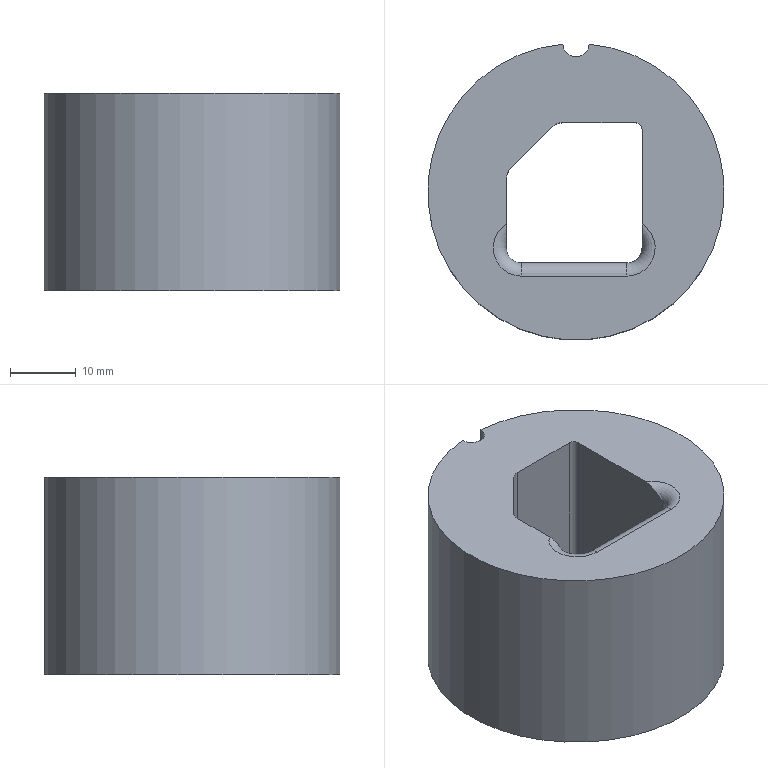Part | NX | features 23 2 | 1 solid | 17 faces | box 45 x 44.911 x 30 mm | volume 35277 mm3 | cylinder 8 | plane 7 | torus 2 | commonest cylinder face diameters 4.6 x4 2 x1 4 x1 4.001 x1 45 x1
STEP:
#1=CARTESIAN_POINT('',(147.222,-436.51,-33.5));
#2=VERTEX_POINT('',#1);
#3=CARTESIAN_POINT('',(144.922,-438.81,-33.5));
#4=VERTEX_POINT('',#3);
#5=CARTESIAN_POINT('',(144.922,-436.51,-33.5));
#6=DIRECTION('',(0.,0.,-1.));
#7=DIRECTION('',(-1.,0.,0.));
#8=AXIS2_PLACEMENT_3D('',#5,#6,#7);
#9=CIRCLE('',#8,2.3);
#10=EDGE_CURVE('',#2,#4,#9,.T.);
#11=ORIENTED_EDGE('',*,*,#10,.F.);
#12=CARTESIAN_POINT('',(147.222,-418.5,-33.5));
#13=VERTEX_POINT('',#12);
#14=CARTESIAN_POINT('',(147.222,-377.506,-33.5));
#15=DIRECTION('',(0.,1.,0.));
#16=VECTOR('',#15,1000.);
#17=LINE('',#14,#16);
#18=EDGE_CURVE('',#2,#13,#17,.T.);
#19=ORIENTED_EDGE('',*,*,#18,.T.);
#20=CARTESIAN_POINT('',(146.222,-417.5,-33.5));
#21=VERTEX_POINT('',#20);
#22=CARTESIAN_POINT('',(146.222,-418.5,-33.5));
#23=DIRECTION('',(0.,0.,1.));
#24=DIRECTION('',(-1.,0.,0.));
#25=AXIS2_PLACEMENT_3D('',#22,#23,#24);
#26=CIRCLE('',#25,1.);
#27=EDGE_CURVE('',#13,#21,#26,.T.);
#28=ORIENTED_EDGE('',*,*,#27,.T.);
#29=CARTESIAN_POINT('',(135.152,-417.5,-33.5));
#30=VERTEX_POINT('',#29);
#31=CARTESIAN_POINT('',(119.455,-417.5,-33.5));
#32=DIRECTION('',(-1.,0.,0.));
#33=VECTOR('',#32,1000.);
#34=LINE('',#31,#33);
#35=EDGE_CURVE('',#21,#30,#34,.T.);
#36=ORIENTED_EDGE('',*,*,#35,.T.);
#37=CARTESIAN_POINT('',(133.525,-418.174,-33.5));
#38=VERTEX_POINT('',#37);
#39=CARTESIAN_POINT('',(135.152,-419.8,-33.5));
#40=DIRECTION('',(0.,0.,1.));
#41=DIRECTION('',(-1.,0.,0.));
#42=AXIS2_PLACEMENT_3D('',#39,#40,#41);
#43=CIRCLE('',#42,2.3);
#44=EDGE_CURVE('',#30,#38,#43,.T.);
#45=ORIENTED_EDGE('',*,*,#44,.T.);
#46=CARTESIAN_POINT('',(127.295,-424.404,-33.5));
#47=VERTEX_POINT('',#46);
#48=CARTESIAN_POINT('',(146.824,-404.875,-33.5));
#49=DIRECTION('',(-0.7071,-0.7071,0.));
#50=VECTOR('',#49,1000.);
#51=LINE('',#48,#50);
#52=EDGE_CURVE('',#38,#47,#51,.T.);
#53=ORIENTED_EDGE('',*,*,#52,.T.);
#54=CARTESIAN_POINT('',(126.622,-426.03,-33.5));
#55=VERTEX_POINT('',#54);
#56=CARTESIAN_POINT('',(128.922,-426.03,-33.5));
#57=DIRECTION('',(0.,0.,1.));
#58=DIRECTION('',(-1.,0.,0.));
#59=AXIS2_PLACEMENT_3D('',#56,#57,#58);
#60=CIRCLE('',#59,2.3);
#61=EDGE_CURVE('',#47,#55,#60,.T.);
#62=ORIENTED_EDGE('',*,*,#61,.T.);
#63=CARTESIAN_POINT('',(126.622,-436.51,-33.5));
#64=VERTEX_POINT('',#63);
#65=CARTESIAN_POINT('',(126.622,-377.506,-33.5));
#66=DIRECTION('',(0.,-1.,0.));
#67=VECTOR('',#66,1000.);
#68=LINE('',#65,#67);
#69=EDGE_CURVE('',#55,#64,#68,.T.);
#70=ORIENTED_EDGE('',*,*,#69,.T.);
#71=CARTESIAN_POINT('',(128.922,-438.81,-33.5));
#72=VERTEX_POINT('',#71);
#73=CARTESIAN_POINT('',(128.922,-436.51,-33.5));
#74=DIRECTION('',(0.,0.,-1.));
#75=DIRECTION('',(-1.,0.,0.));
#76=AXIS2_PLACEMENT_3D('',#73,#74,#75);
#77=CIRCLE('',#76,2.3);
#78=EDGE_CURVE('',#72,#64,#77,.T.);
#79=ORIENTED_EDGE('',*,*,#78,.F.);
#80=CARTESIAN_POINT('',(119.455,-438.81,-33.5));
#81=DIRECTION('',(1.,0.,0.));
#82=VECTOR('',#81,1000.);
#83=LINE('',#80,#82);
#84=EDGE_CURVE('',#72,#4,#83,.T.);
#85=ORIENTED_EDGE('',*,*,#84,.T.);
#86=EDGE_LOOP('',(#11,#19,#28,#36,#45,#53,#62,#70,#79,#85));
#87=FACE_BOUND('',#86,.T.);
#88=CARTESIAN_POINT('',(139.198,-405.589,-33.5));
#89=VERTEX_POINT('',#88);
#90=CARTESIAN_POINT('',(135.201,-405.589,-33.5));
#91=VERTEX_POINT('',#90);
#92=CARTESIAN_POINT('',(137.199,-428.,-33.5));
#93=DIRECTION('',(0.,0.,-1.));
#94=DIRECTION('',(-1.,0.,0.));
#95=AXIS2_PLACEMENT_3D('',#92,#93,#94);
#96=CIRCLE('',#95,22.5);
#97=EDGE_CURVE('',#89,#91,#96,.T.);
#98=ORIENTED_EDGE('',*,*,#97,.T.);
#99=CARTESIAN_POINT('',(137.199,-405.5,-33.5));
#100=DIRECTION('',(0.,0.,1.));
#101=DIRECTION('',(1.,0.,0.));
#102=AXIS2_PLACEMENT_3D('',#99,#100,#101);
#103=CIRCLE('',#102,2.001);
#104=EDGE_CURVE('',#91,#89,#103,.T.);
#105=ORIENTED_EDGE('',*,*,#104,.T.);
#106=EDGE_LOOP('',(#98,#105));
#107=FACE_BOUND('',#106,.T.);
#108=CARTESIAN_POINT('',(119.455,-377.506,-33.5));
#109=DIRECTION('',(0.,0.,-1.));
#110=DIRECTION('',(-1.,0.,0.));
#111=AXIS2_PLACEMENT_3D('',#108,#109,#110);
#112=PLANE('',#111);
#113=ADVANCED_FACE('',(#87,#107),#112,.T.);
#114=CARTESIAN_POINT('',(135.201,-405.589,-3.5));
#115=VERTEX_POINT('',#114);
#116=CARTESIAN_POINT('',(139.198,-405.589,-3.5));
#117=VERTEX_POINT('',#116);
#118=CARTESIAN_POINT('',(137.199,-428.,-3.5));
#119=DIRECTION('',(0.,0.,1.));
#120=DIRECTION('',(-1.,0.,0.));
#121=AXIS2_PLACEMENT_3D('',#118,#119,#120);
#122=CIRCLE('',#121,22.5);
#123=EDGE_CURVE('',#115,#117,#122,.T.);
#124=ORIENTED_EDGE('',*,*,#123,.F.);
#125=CARTESIAN_POINT('',(135.201,-405.589,66.5));
#126=DIRECTION('',(0.,0.,-1.));
#127=VECTOR('',#126,1000.);
#128=LINE('',#125,#127);
#129=EDGE_CURVE('',#115,#91,#128,.T.);
#130=ORIENTED_EDGE('',*,*,#129,.T.);
#131=ORIENTED_EDGE('',*,*,#97,.F.);
#132=CARTESIAN_POINT('',(139.198,-405.589,66.5));
#133=DIRECTION('',(0.,0.,1.));
#134=VECTOR('',#133,1000.);
#135=LINE('',#132,#134);
#136=EDGE_CURVE('',#89,#117,#135,.T.);
#137=ORIENTED_EDGE('',*,*,#136,.T.);
#138=EDGE_LOOP('',(#124,#130,#131,#137));
#139=FACE_BOUND('',#138,.T.);
#140=CARTESIAN_POINT('',(137.199,-428.,-158.));
#141=DIRECTION('',(0.,0.,1.));
#142=DIRECTION('',(-1.,0.,0.));
#143=AXIS2_PLACEMENT_3D('',#140,#141,#142);
#144=CYLINDRICAL_SURFACE('',#143,22.5);
#145=ADVANCED_FACE('',(#139),#144,.T.);
#146=CARTESIAN_POINT('',(147.222,-436.51,-5.5));
#147=VERTEX_POINT('',#146);
#148=CARTESIAN_POINT('',(147.222,-436.51,210.5));
#149=DIRECTION('',(0.,0.,1.));
#150=VECTOR('',#149,1000.);
#151=LINE('',#148,#150);
#152=EDGE_CURVE('',#2,#147,#151,.T.);
#153=ORIENTED_EDGE('',*,*,#152,.T.);
#154=CARTESIAN_POINT('',(147.222,-432.877,-3.5));
#155=VERTEX_POINT('',#154);
#156=CARTESIAN_POINT('',(147.222,-436.51,-5.5));
#157=CARTESIAN_POINT('',(147.222,-435.992,-5.017));
#158=CARTESIAN_POINT('',(147.222,-434.95,-4.041));
#159=CARTESIAN_POINT('',(147.222,-433.59,-3.5));
#160=CARTESIAN_POINT('',(147.222,-432.877,-3.5));
#161=B_SPLINE_CURVE_WITH_KNOTS('',3,(#156,#157,#158,#159,#160),.UNSPECIFIED.,.F.,.F.,(4,1,4),(-0.000009592,0.002115,0.004239),.UNSPECIFIED.);
#162=EDGE_CURVE('',#147,#155,#161,.T.);
#163=ORIENTED_EDGE('',*,*,#162,.T.);
#164=CARTESIAN_POINT('',(147.222,-418.5,-3.5));
#165=VERTEX_POINT('',#164);
#166=CARTESIAN_POINT('',(147.222,-384.125,-3.5));
#167=DIRECTION('',(0.,-1.,0.));
#168=VECTOR('',#167,1000.);
#169=LINE('',#166,#168);
#170=EDGE_CURVE('',#165,#155,#169,.T.);
#171=ORIENTED_EDGE('',*,*,#170,.F.);
#172=CARTESIAN_POINT('',(147.222,-418.5,210.5));
#173=DIRECTION('',(0.,0.,1.));
#174=VECTOR('',#173,1000.);
#175=LINE('',#172,#174);
#176=EDGE_CURVE('',#13,#165,#175,.T.);
#177=ORIENTED_EDGE('',*,*,#176,.F.);
#178=ORIENTED_EDGE('',*,*,#18,.F.);
#179=EDGE_LOOP('',(#153,#163,#171,#177,#178));
#180=FACE_BOUND('',#179,.T.);
#181=CARTESIAN_POINT('',(147.222,-384.125,210.5));
#182=DIRECTION('',(-1.,0.,0.));
#183=DIRECTION('',(0.,0.,1.));
#184=AXIS2_PLACEMENT_3D('',#181,#182,#183);
#185=PLANE('',#184);
#186=ADVANCED_FACE('',(#180),#185,.T.);
#187=CARTESIAN_POINT('',(146.222,-417.5,-3.5));
#188=VERTEX_POINT('',#187);
#189=CARTESIAN_POINT('',(146.222,-417.5,210.5));
#190=DIRECTION('',(0.,0.,1.));
#191=VECTOR('',#190,1000.);
#192=LINE('',#189,#191);
#193=EDGE_CURVE('',#21,#188,#192,.T.);
#194=ORIENTED_EDGE('',*,*,#193,.F.);
#195=ORIENTED_EDGE('',*,*,#27,.F.);
#196=ORIENTED_EDGE('',*,*,#176,.T.);
#197=CARTESIAN_POINT('',(146.222,-418.5,-3.5));
#198=DIRECTION('',(0.,0.,-1.));
#199=DIRECTION('',(-1.,0.,0.));
#200=AXIS2_PLACEMENT_3D('',#197,#198,#199);
#201=CIRCLE('',#200,1.);
#202=EDGE_CURVE('',#188,#165,#201,.T.);
#203=ORIENTED_EDGE('',*,*,#202,.F.);
#204=EDGE_LOOP('',(#194,#195,#196,#203));
#205=FACE_BOUND('',#204,.T.);
#206=CARTESIAN_POINT('',(146.222,-418.5,210.5));
#207=DIRECTION('',(0.,0.,-1.));
#208=DIRECTION('',(1.,0.,0.));
#209=AXIS2_PLACEMENT_3D('',#206,#207,#208);
#210=CYLINDRICAL_SURFACE('',#209,1.);
#211=ADVANCED_FACE('',(#205),#210,.F.);
#212=CARTESIAN_POINT('',(135.152,-417.5,-3.5));
#213=VERTEX_POINT('',#212);
#214=CARTESIAN_POINT('',(135.152,-417.5,210.5));
#215=DIRECTION('',(0.,0.,1.));
#216=VECTOR('',#215,1000.);
#217=LINE('',#214,#216);
#218=EDGE_CURVE('',#30,#213,#217,.T.);
#219=ORIENTED_EDGE('',*,*,#218,.F.);
#220=ORIENTED_EDGE('',*,*,#35,.F.);
#221=ORIENTED_EDGE('',*,*,#193,.T.);
#222=CARTESIAN_POINT('',(205.494,-417.5,-3.5));
#223=DIRECTION('',(1.,0.,0.));
#224=VECTOR('',#223,1000.);
#225=LINE('',#222,#224);
#226=EDGE_CURVE('',#213,#188,#225,.T.);
#227=ORIENTED_EDGE('',*,*,#226,.F.);
#228=EDGE_LOOP('',(#219,#220,#221,#227));
#229=FACE_BOUND('',#228,.T.);
#230=CARTESIAN_POINT('',(205.494,-417.5,210.5));
#231=DIRECTION('',(0.,-1.,0.));
#232=DIRECTION('',(0.,0.,-1.));
#233=AXIS2_PLACEMENT_3D('',#230,#231,#232);
#234=PLANE('',#233);
#235=ADVANCED_FACE('',(#229),#234,.T.);
#236=CARTESIAN_POINT('',(133.525,-418.174,-3.5));
#237=VERTEX_POINT('',#236);
#238=CARTESIAN_POINT('',(133.525,-418.174,-48.5));
#239=DIRECTION('',(0.,0.,1.));
#240=VECTOR('',#239,1000.);
#241=LINE('',#238,#240);
#242=EDGE_CURVE('',#38,#237,#241,.T.);
#243=ORIENTED_EDGE('',*,*,#242,.F.);
#244=ORIENTED_EDGE('',*,*,#44,.F.);
#245=ORIENTED_EDGE('',*,*,#218,.T.);
#246=CARTESIAN_POINT('',(135.152,-419.8,-3.5));
#247=DIRECTION('',(0.,0.,-1.));
#248=DIRECTION('',(-1.,0.,0.));
#249=AXIS2_PLACEMENT_3D('',#246,#247,#248);
#250=CIRCLE('',#249,2.3);
#251=EDGE_CURVE('',#237,#213,#250,.T.);
#252=ORIENTED_EDGE('',*,*,#251,.F.);
#253=EDGE_LOOP('',(#243,#244,#245,#252));
#254=FACE_BOUND('',#253,.T.);
#255=CARTESIAN_POINT('',(135.152,-419.8,-48.5));
#256=DIRECTION('',(0.,0.,-1.));
#257=DIRECTION('',(1.,0.,0.));
#258=AXIS2_PLACEMENT_3D('',#255,#256,#257);
#259=CYLINDRICAL_SURFACE('',#258,2.3);
#260=ADVANCED_FACE('',(#254),#259,.F.);
#261=CARTESIAN_POINT('',(127.295,-424.404,-3.5));
#262=VERTEX_POINT('',#261);
#263=CARTESIAN_POINT('',(127.295,-424.404,-48.5));
#264=DIRECTION('',(0.,0.,1.));
#265=VECTOR('',#264,1000.);
#266=LINE('',#263,#265);
#267=EDGE_CURVE('',#47,#262,#266,.T.);
#268=ORIENTED_EDGE('',*,*,#267,.F.);
#269=ORIENTED_EDGE('',*,*,#52,.F.);
#270=ORIENTED_EDGE('',*,*,#242,.T.);
#271=CARTESIAN_POINT('',(127.785,-423.914,-3.5));
#272=DIRECTION('',(0.7071,0.7071,0.));
#273=VECTOR('',#272,1000.);
#274=LINE('',#271,#273);
#275=EDGE_CURVE('',#262,#237,#274,.T.);
#276=ORIENTED_EDGE('',*,*,#275,.F.);
#277=EDGE_LOOP('',(#268,#269,#270,#276));
#278=FACE_BOUND('',#277,.T.);
#279=CARTESIAN_POINT('',(127.785,-423.914,-48.5));
#280=DIRECTION('',(0.7071,-0.7071,0.));
#281=DIRECTION('',(0.7071,0.7071,0.));
#282=AXIS2_PLACEMENT_3D('',#279,#280,#281);
#283=PLANE('',#282);
#284=ADVANCED_FACE('',(#278),#283,.T.);
#285=CARTESIAN_POINT('',(126.622,-426.03,-3.5));
#286=VERTEX_POINT('',#285);
#287=CARTESIAN_POINT('',(126.622,-426.03,210.5));
#288=DIRECTION('',(0.,0.,1.));
#289=VECTOR('',#288,1000.);
#290=LINE('',#287,#289);
#291=EDGE_CURVE('',#55,#286,#290,.T.);
#292=ORIENTED_EDGE('',*,*,#291,.F.);
#293=ORIENTED_EDGE('',*,*,#61,.F.);
#294=ORIENTED_EDGE('',*,*,#267,.T.);
#295=CARTESIAN_POINT('',(128.922,-426.03,-3.5));
#296=DIRECTION('',(0.,0.,-1.));
#297=DIRECTION('',(-1.,0.,0.));
#298=AXIS2_PLACEMENT_3D('',#295,#296,#297);
#299=CIRCLE('',#298,2.3);
#300=EDGE_CURVE('',#286,#262,#299,.T.);
#301=ORIENTED_EDGE('',*,*,#300,.F.);
#302=EDGE_LOOP('',(#292,#293,#294,#301));
#303=FACE_BOUND('',#302,.T.);
#304=CARTESIAN_POINT('',(128.922,-426.03,210.5));
#305=DIRECTION('',(0.,0.,-1.));
#306=DIRECTION('',(1.,0.,0.));
#307=AXIS2_PLACEMENT_3D('',#304,#305,#306);
#308=CYLINDRICAL_SURFACE('',#307,2.3);
#309=ADVANCED_FACE('',(#303),#308,.F.);
#310=CARTESIAN_POINT('',(126.622,-432.877,-3.5));
#311=VERTEX_POINT('',#310);
#312=CARTESIAN_POINT('',(126.622,-384.125,-3.5));
#313=DIRECTION('',(0.,1.,0.));
#314=VECTOR('',#313,1000.);
#315=LINE('',#312,#314);
#316=EDGE_CURVE('',#311,#286,#315,.T.);
#317=ORIENTED_EDGE('',*,*,#316,.F.);
#318=CARTESIAN_POINT('',(126.622,-436.51,-5.5));
#319=VERTEX_POINT('',#318);
#320=CARTESIAN_POINT('',(126.622,-432.877,-3.5));
#321=CARTESIAN_POINT('',(126.622,-433.593,-3.5));
#322=CARTESIAN_POINT('',(126.622,-434.946,-4.04));
#323=CARTESIAN_POINT('',(126.622,-435.993,-5.018));
#324=CARTESIAN_POINT('',(126.622,-436.51,-5.5));
#325=B_SPLINE_CURVE_WITH_KNOTS('',3,(#320,#321,#322,#323,#324),.UNSPECIFIED.,.F.,.F.,(4,1,4),(0.,0.00212,0.00424),.UNSPECIFIED.);
#326=EDGE_CURVE('',#311,#319,#325,.T.);
#327=ORIENTED_EDGE('',*,*,#326,.T.);
#328=CARTESIAN_POINT('',(126.622,-436.51,210.5));
#329=DIRECTION('',(0.,0.,1.));
#330=VECTOR('',#329,1000.);
#331=LINE('',#328,#330);
#332=EDGE_CURVE('',#64,#319,#331,.T.);
#333=ORIENTED_EDGE('',*,*,#332,.F.);
#334=ORIENTED_EDGE('',*,*,#69,.F.);
#335=ORIENTED_EDGE('',*,*,#291,.T.);
#336=EDGE_LOOP('',(#317,#327,#333,#334,#335));
#337=FACE_BOUND('',#336,.T.);
#338=CARTESIAN_POINT('',(126.622,-384.125,210.5));
#339=DIRECTION('',(1.,0.,0.));
#340=DIRECTION('',(0.,0.,-1.));
#341=AXIS2_PLACEMENT_3D('',#338,#339,#340);
#342=PLANE('',#341);
#343=ADVANCED_FACE('',(#337),#342,.T.);
#344=ORIENTED_EDGE('',*,*,#170,.T.);
#345=CARTESIAN_POINT('',(144.922,-440.81,-3.5));
#346=VERTEX_POINT('',#345);
#347=CARTESIAN_POINT('',(144.922,-436.51,-3.5));
#348=DIRECTION('',(0.,0.,-1.));
#349=DIRECTION('',(-1.,0.,0.));
#350=AXIS2_PLACEMENT_3D('',#347,#348,#349);
#351=CIRCLE('',#350,4.3);
#352=EDGE_CURVE('',#155,#346,#351,.T.);
#353=ORIENTED_EDGE('',*,*,#352,.T.);
#354=CARTESIAN_POINT('',(128.922,-440.81,-3.5));
#355=VERTEX_POINT('',#354);
#356=CARTESIAN_POINT('',(128.922,-440.81,-3.5));
#357=DIRECTION('',(-1.,0.,0.));
#358=VECTOR('',#357,1000.);
#359=LINE('',#356,#358);
#360=EDGE_CURVE('',#346,#355,#359,.T.);
#361=ORIENTED_EDGE('',*,*,#360,.T.);
#362=CARTESIAN_POINT('',(128.922,-436.51,-3.5));
#363=DIRECTION('',(0.,0.,-1.));
#364=DIRECTION('',(-1.,0.,0.));
#365=AXIS2_PLACEMENT_3D('',#362,#363,#364);
#366=CIRCLE('',#365,4.3);
#367=EDGE_CURVE('',#355,#311,#366,.T.);
#368=ORIENTED_EDGE('',*,*,#367,.T.);
#369=ORIENTED_EDGE('',*,*,#316,.T.);
#370=ORIENTED_EDGE('',*,*,#300,.T.);
#371=ORIENTED_EDGE('',*,*,#275,.T.);
#372=ORIENTED_EDGE('',*,*,#251,.T.);
#373=ORIENTED_EDGE('',*,*,#226,.T.);
#374=ORIENTED_EDGE('',*,*,#202,.T.);
#375=EDGE_LOOP('',(#344,#353,#361,#368,#369,#370,#371,#372,#373,#374));
#376=FACE_BOUND('',#375,.T.);
#377=ORIENTED_EDGE('',*,*,#123,.T.);
#378=CARTESIAN_POINT('',(137.199,-405.5,-3.5));
#379=DIRECTION('',(0.,0.,-1.));
#380=DIRECTION('',(-1.,0.,0.));
#381=AXIS2_PLACEMENT_3D('',#378,#379,#380);
#382=CIRCLE('',#381,2.001);
#383=EDGE_CURVE('',#117,#115,#382,.T.);
#384=ORIENTED_EDGE('',*,*,#383,.T.);
#385=EDGE_LOOP('',(#377,#384));
#386=FACE_BOUND('',#385,.T.);
#387=CARTESIAN_POINT('',(205.494,-384.125,-3.5));
#388=DIRECTION('',(0.,0.,-1.));
#389=DIRECTION('',(-1.,0.,0.));
#390=AXIS2_PLACEMENT_3D('',#387,#388,#389);
#391=PLANE('',#390);
#392=ADVANCED_FACE('',(#376,#386),#391,.F.);
#393=CARTESIAN_POINT('',(144.922,-438.81,-5.5));
#394=VERTEX_POINT('',#393);
#395=CARTESIAN_POINT('',(144.922,-438.81,210.5));
#396=DIRECTION('',(0.,0.,1.));
#397=VECTOR('',#396,1000.);
#398=LINE('',#395,#397);
#399=EDGE_CURVE('',#4,#394,#398,.T.);
#400=ORIENTED_EDGE('',*,*,#399,.T.);
#401=CARTESIAN_POINT('',(144.922,-436.51,-5.5));
#402=DIRECTION('',(0.,0.,1.));
#403=DIRECTION('',(-1.,0.,0.));
#404=AXIS2_PLACEMENT_3D('',#401,#402,#403);
#405=CIRCLE('',#404,2.3);
#406=EDGE_CURVE('',#394,#147,#405,.T.);
#407=ORIENTED_EDGE('',*,*,#406,.T.);
#408=ORIENTED_EDGE('',*,*,#152,.F.);
#409=ORIENTED_EDGE('',*,*,#10,.T.);
#410=EDGE_LOOP('',(#400,#407,#408,#409));
#411=FACE_BOUND('',#410,.T.);
#412=CARTESIAN_POINT('',(144.922,-436.51,210.5));
#413=DIRECTION('',(0.,0.,-1.));
#414=DIRECTION('',(1.,0.,0.));
#415=AXIS2_PLACEMENT_3D('',#412,#413,#414);
#416=CYLINDRICAL_SURFACE('',#415,2.3);
#417=ADVANCED_FACE('',(#411),#416,.F.);
#418=CARTESIAN_POINT('',(128.922,-438.81,-5.5));
#419=VERTEX_POINT('',#418);
#420=CARTESIAN_POINT('',(128.922,-438.81,210.5));
#421=DIRECTION('',(0.,0.,1.));
#422=VECTOR('',#421,1000.);
#423=LINE('',#420,#422);
#424=EDGE_CURVE('',#72,#419,#423,.T.);
#425=ORIENTED_EDGE('',*,*,#424,.T.);
#426=CARTESIAN_POINT('',(144.922,-438.81,-5.5));
#427=DIRECTION('',(1.,0.,0.));
#428=VECTOR('',#427,1000.);
#429=LINE('',#426,#428);
#430=EDGE_CURVE('',#419,#394,#429,.T.);
#431=ORIENTED_EDGE('',*,*,#430,.T.);
#432=ORIENTED_EDGE('',*,*,#399,.F.);
#433=ORIENTED_EDGE('',*,*,#84,.F.);
#434=EDGE_LOOP('',(#425,#431,#432,#433));
#435=FACE_BOUND('',#434,.T.);
#436=CARTESIAN_POINT('',(205.494,-438.81,210.5));
#437=DIRECTION('',(0.,1.,0.));
#438=DIRECTION('',(0.,0.,1.));
#439=AXIS2_PLACEMENT_3D('',#436,#437,#438);
#440=PLANE('',#439);
#441=ADVANCED_FACE('',(#435),#440,.T.);
#442=ORIENTED_EDGE('',*,*,#332,.T.);
#443=CARTESIAN_POINT('',(128.922,-436.51,-5.5));
#444=DIRECTION('',(0.,0.,1.));
#445=DIRECTION('',(-1.,0.,0.));
#446=AXIS2_PLACEMENT_3D('',#443,#444,#445);
#447=CIRCLE('',#446,2.3);
#448=EDGE_CURVE('',#319,#419,#447,.T.);
#449=ORIENTED_EDGE('',*,*,#448,.T.);
#450=ORIENTED_EDGE('',*,*,#424,.F.);
#451=ORIENTED_EDGE('',*,*,#78,.T.);
#452=EDGE_LOOP('',(#442,#449,#450,#451));
#453=FACE_BOUND('',#452,.T.);
#454=CARTESIAN_POINT('',(128.922,-436.51,210.5));
#455=DIRECTION('',(0.,0.,-1.));
#456=DIRECTION('',(1.,0.,0.));
#457=AXIS2_PLACEMENT_3D('',#454,#455,#456);
#458=CYLINDRICAL_SURFACE('',#457,2.3);
#459=ADVANCED_FACE('',(#453),#458,.F.);
#460=ORIENTED_EDGE('',*,*,#383,.F.);
#461=ORIENTED_EDGE('',*,*,#136,.F.);
#462=ORIENTED_EDGE('',*,*,#104,.F.);
#463=ORIENTED_EDGE('',*,*,#129,.F.);
#464=EDGE_LOOP('',(#460,#461,#462,#463));
#465=FACE_BOUND('',#464,.T.);
#466=CARTESIAN_POINT('',(137.199,-405.5,-33.5));
#467=DIRECTION('',(0.,0.,1.));
#468=DIRECTION('',(-1.,0.,0.));
#469=AXIS2_PLACEMENT_3D('',#466,#467,#468);
#470=CYLINDRICAL_SURFACE('',#469,2.001);
#471=ADVANCED_FACE('',(#465),#470,.F.);
#472=ORIENTED_EDGE('',*,*,#326,.F.);
#473=ORIENTED_EDGE('',*,*,#367,.F.);
#474=CARTESIAN_POINT('',(128.922,-440.81,-5.5));
#475=DIRECTION('',(1.,0.,0.));
#476=DIRECTION('',(0.,0.,-1.));
#477=AXIS2_PLACEMENT_3D('',#474,#475,#476);
#478=CIRCLE('',#477,2.);
#479=EDGE_CURVE('',#419,#355,#478,.T.);
#480=ORIENTED_EDGE('',*,*,#479,.F.);
#481=ORIENTED_EDGE('',*,*,#448,.F.);
#482=EDGE_LOOP('',(#472,#473,#480,#481));
#483=FACE_BOUND('',#482,.T.);
#484=CARTESIAN_POINT('',(128.922,-436.51,-5.5));
#485=DIRECTION('',(0.,0.,-1.));
#486=DIRECTION('',(1.,0.,0.));
#487=AXIS2_PLACEMENT_3D('',#484,#485,#486);
#488=TOROIDAL_SURFACE('',#487,4.3,2.);
#489=ADVANCED_FACE('',(#483),#488,.T.);
#490=ORIENTED_EDGE('',*,*,#479,.T.);
#491=ORIENTED_EDGE('',*,*,#360,.F.);
#492=CARTESIAN_POINT('',(144.922,-440.81,-5.5));
#493=DIRECTION('',(1.,0.,0.));
#494=DIRECTION('',(0.,0.,-1.));
#495=AXIS2_PLACEMENT_3D('',#492,#493,#494);
#496=CIRCLE('',#495,2.);
#497=EDGE_CURVE('',#394,#346,#496,.T.);
#498=ORIENTED_EDGE('',*,*,#497,.F.);
#499=ORIENTED_EDGE('',*,*,#430,.F.);
#500=EDGE_LOOP('',(#490,#491,#498,#499));
#501=FACE_BOUND('',#500,.T.);
#502=CARTESIAN_POINT('',(205.494,-440.81,-5.5));
#503=DIRECTION('',(-1.,0.,0.));
#504=DIRECTION('',(0.,0.,-1.));
#505=AXIS2_PLACEMENT_3D('',#502,#503,#504);
#506=CYLINDRICAL_SURFACE('',#505,2.);
#507=ADVANCED_FACE('',(#501),#506,.T.);
#508=ORIENTED_EDGE('',*,*,#497,.T.);
#509=ORIENTED_EDGE('',*,*,#352,.F.);
#510=ORIENTED_EDGE('',*,*,#162,.F.);
#511=ORIENTED_EDGE('',*,*,#406,.F.);
#512=EDGE_LOOP('',(#508,#509,#510,#511));
#513=FACE_BOUND('',#512,.T.);
#514=CARTESIAN_POINT('',(144.922,-436.51,-5.5));
#515=DIRECTION('',(0.,0.,-1.));
#516=DIRECTION('',(1.,0.,0.));
#517=AXIS2_PLACEMENT_3D('',#514,#515,#516);
#518=TOROIDAL_SURFACE('',#517,4.3,2.);
#519=ADVANCED_FACE('',(#513),#518,.T.);
#520=CLOSED_SHELL('',(#113,#145,#186,#211,#235,#260,#284,#309,#343,#392,#417,#441,#459,#471,#489,#507,#519));
#521=MANIFOLD_SOLID_BREP('',#520);
#522=(LENGTH_UNIT()NAMED_UNIT(*)SI_UNIT(.MILLI.,.METRE.));
#523=UNCERTAINTY_MEASURE_WITH_UNIT(LENGTH_MEASURE(0.0508),#522,'','');
#524=(NAMED_UNIT(*)PLANE_ANGLE_UNIT()SI_UNIT($,.RADIAN.));
#525=(NAMED_UNIT(*)SI_UNIT($,.STERADIAN.)SOLID_ANGLE_UNIT());
#526=(GEOMETRIC_REPRESENTATION_CONTEXT(3)GLOBAL_UNCERTAINTY_ASSIGNED_CONTEXT((#523))GLOBAL_UNIT_ASSIGNED_CONTEXT((#522,#524,#525))REPRESENTATION_CONTEXT('',''));
#527=ADVANCED_BREP_SHAPE_REPRESENTATION('',(#521),#526);